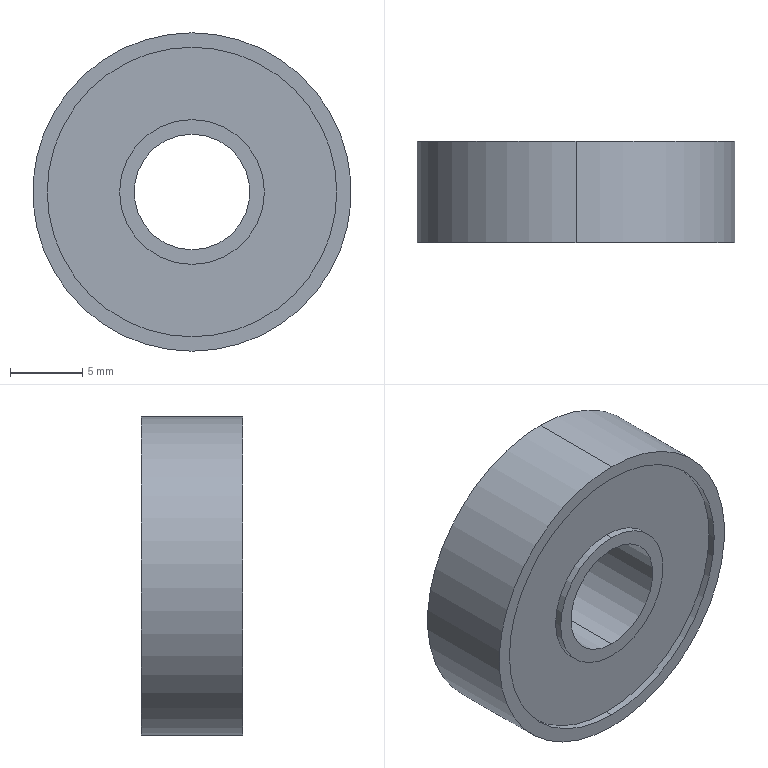Part | SolidWorks | features ICE 2, Extrusion 1 | 1 solid | 18 faces | box 22 x 7 x 22 mm | volume 2073 mm3 | cylinder 12 | plane 6 | commonest cylinder face diameters 10 x4 20 x4 8 x2 22 x2
STEP:
#1=CARTESIAN_POINT('',(0.,6.5,5.));
#2=VERTEX_POINT('',#1);
#3=CARTESIAN_POINT('',(0.,6.5,-5.));
#4=VERTEX_POINT('',#3);
#5=CARTESIAN_POINT('',(0.,6.5,0.));
#6=DIRECTION('',(0.,1.,0.));
#7=DIRECTION('',(0.,0.,1.));
#8=AXIS2_PLACEMENT_3D('',#5,#6,#7);
#9=CIRCLE('',#8,5.);
#10=EDGE_CURVE('',#2,#4,#9,.T.);
#11=ORIENTED_EDGE('',*,*,#10,.T.);
#12=CARTESIAN_POINT('',(0.,7.,-5.));
#13=VERTEX_POINT('',#12);
#14=CARTESIAN_POINT('',(0.,6.5,-5.));
#15=DIRECTION('',(0.,1.,0.));
#16=VECTOR('',#15,1000.);
#17=LINE('',#14,#16);
#18=EDGE_CURVE('',#4,#13,#17,.T.);
#19=ORIENTED_EDGE('',*,*,#18,.T.);
#20=CARTESIAN_POINT('',(0.,7.,5.));
#21=VERTEX_POINT('',#20);
#22=CARTESIAN_POINT('',(0.,7.,0.));
#23=DIRECTION('',(0.,1.,0.));
#24=DIRECTION('',(0.,0.,1.));
#25=AXIS2_PLACEMENT_3D('',#22,#23,#24);
#26=CIRCLE('',#25,5.);
#27=EDGE_CURVE('',#21,#13,#26,.T.);
#28=ORIENTED_EDGE('',*,*,#27,.F.);
#29=CARTESIAN_POINT('',(0.,6.5,5.));
#30=DIRECTION('',(0.,1.,0.));
#31=VECTOR('',#30,1000.);
#32=LINE('',#29,#31);
#33=EDGE_CURVE('',#2,#21,#32,.T.);
#34=ORIENTED_EDGE('',*,*,#33,.F.);
#35=EDGE_LOOP('',(#11,#19,#28,#34));
#36=FACE_OUTER_BOUND('',#35,.T.);
#37=CARTESIAN_POINT('',(0.,6.5,0.));
#38=DIRECTION('',(0.,1.,0.));
#39=DIRECTION('',(0.,0.,1.));
#40=AXIS2_PLACEMENT_3D('',#37,#38,#39);
#41=CYLINDRICAL_SURFACE('',#40,5.);
#42=ADVANCED_FACE('',(#36),#41,.T.);
#43=CARTESIAN_POINT('',(0.,6.5,-10.));
#44=VERTEX_POINT('',#43);
#45=CARTESIAN_POINT('',(0.,6.5,10.));
#46=VERTEX_POINT('',#45);
#47=CARTESIAN_POINT('',(0.,6.5,0.));
#48=DIRECTION('',(0.,1.,0.));
#49=DIRECTION('',(0.,0.,1.));
#50=AXIS2_PLACEMENT_3D('',#47,#48,#49);
#51=CIRCLE('',#50,10.);
#52=EDGE_CURVE('',#44,#46,#51,.T.);
#53=ORIENTED_EDGE('',*,*,#52,.F.);
#54=CARTESIAN_POINT('',(0.,7.,-10.));
#55=VERTEX_POINT('',#54);
#56=CARTESIAN_POINT('',(0.,6.5,-10.));
#57=DIRECTION('',(0.,1.,0.));
#58=VECTOR('',#57,1000.);
#59=LINE('',#56,#58);
#60=EDGE_CURVE('',#44,#55,#59,.T.);
#61=ORIENTED_EDGE('',*,*,#60,.T.);
#62=CARTESIAN_POINT('',(0.,7.,10.));
#63=VERTEX_POINT('',#62);
#64=CARTESIAN_POINT('',(0.,7.,0.));
#65=DIRECTION('',(0.,1.,0.));
#66=DIRECTION('',(0.,0.,1.));
#67=AXIS2_PLACEMENT_3D('',#64,#65,#66);
#68=CIRCLE('',#67,10.);
#69=EDGE_CURVE('',#55,#63,#68,.T.);
#70=ORIENTED_EDGE('',*,*,#69,.T.);
#71=CARTESIAN_POINT('',(0.,6.5,10.));
#72=DIRECTION('',(0.,1.,0.));
#73=VECTOR('',#72,1000.);
#74=LINE('',#71,#73);
#75=EDGE_CURVE('',#46,#63,#74,.T.);
#76=ORIENTED_EDGE('',*,*,#75,.F.);
#77=EDGE_LOOP('',(#53,#61,#70,#76));
#78=FACE_OUTER_BOUND('',#77,.T.);
#79=CARTESIAN_POINT('',(0.,6.5,0.));
#80=DIRECTION('',(0.,1.,0.));
#81=DIRECTION('',(0.,0.,1.));
#82=AXIS2_PLACEMENT_3D('',#79,#80,#81);
#83=CYLINDRICAL_SURFACE('',#82,10.);
#84=ADVANCED_FACE('',(#78),#83,.F.);
#85=CARTESIAN_POINT('',(0.,0.5,-5.));
#86=VERTEX_POINT('',#85);
#87=CARTESIAN_POINT('',(0.,0.5,5.));
#88=VERTEX_POINT('',#87);
#89=CARTESIAN_POINT('',(0.,0.5,0.));
#90=DIRECTION('',(0.,-1.,0.));
#91=DIRECTION('',(0.,0.,-1.));
#92=AXIS2_PLACEMENT_3D('',#89,#90,#91);
#93=CIRCLE('',#92,5.);
#94=EDGE_CURVE('',#86,#88,#93,.T.);
#95=ORIENTED_EDGE('',*,*,#94,.T.);
#96=CARTESIAN_POINT('',(0.,0.,5.));
#97=VERTEX_POINT('',#96);
#98=CARTESIAN_POINT('',(0.,0.5,5.));
#99=DIRECTION('',(0.,-1.,0.));
#100=VECTOR('',#99,1000.);
#101=LINE('',#98,#100);
#102=EDGE_CURVE('',#88,#97,#101,.T.);
#103=ORIENTED_EDGE('',*,*,#102,.T.);
#104=CARTESIAN_POINT('',(0.,0.,-5.));
#105=VERTEX_POINT('',#104);
#106=CARTESIAN_POINT('',(0.,0.,0.));
#107=DIRECTION('',(0.,-1.,0.));
#108=DIRECTION('',(0.,0.,-1.));
#109=AXIS2_PLACEMENT_3D('',#106,#107,#108);
#110=CIRCLE('',#109,5.);
#111=EDGE_CURVE('',#105,#97,#110,.T.);
#112=ORIENTED_EDGE('',*,*,#111,.F.);
#113=CARTESIAN_POINT('',(0.,0.5,-5.));
#114=DIRECTION('',(0.,-1.,0.));
#115=VECTOR('',#114,1000.);
#116=LINE('',#113,#115);
#117=EDGE_CURVE('',#86,#105,#116,.T.);
#118=ORIENTED_EDGE('',*,*,#117,.F.);
#119=EDGE_LOOP('',(#95,#103,#112,#118));
#120=FACE_OUTER_BOUND('',#119,.T.);
#121=CARTESIAN_POINT('',(0.,0.5,0.));
#122=DIRECTION('',(0.,-1.,0.));
#123=DIRECTION('',(0.,0.,-1.));
#124=AXIS2_PLACEMENT_3D('',#121,#122,#123);
#125=CYLINDRICAL_SURFACE('',#124,5.);
#126=ADVANCED_FACE('',(#120),#125,.T.);
#127=CARTESIAN_POINT('',(0.,0.5,10.));
#128=VERTEX_POINT('',#127);
#129=CARTESIAN_POINT('',(0.,0.5,-10.));
#130=VERTEX_POINT('',#129);
#131=CARTESIAN_POINT('',(0.,0.5,0.));
#132=DIRECTION('',(0.,-1.,0.));
#133=DIRECTION('',(0.,0.,-1.));
#134=AXIS2_PLACEMENT_3D('',#131,#132,#133);
#135=CIRCLE('',#134,10.);
#136=EDGE_CURVE('',#128,#130,#135,.T.);
#137=ORIENTED_EDGE('',*,*,#136,.F.);
#138=CARTESIAN_POINT('',(0.,0.,10.));
#139=VERTEX_POINT('',#138);
#140=CARTESIAN_POINT('',(0.,0.5,10.));
#141=DIRECTION('',(0.,-1.,0.));
#142=VECTOR('',#141,1000.);
#143=LINE('',#140,#142);
#144=EDGE_CURVE('',#128,#139,#143,.T.);
#145=ORIENTED_EDGE('',*,*,#144,.T.);
#146=CARTESIAN_POINT('',(0.,0.,-10.));
#147=VERTEX_POINT('',#146);
#148=CARTESIAN_POINT('',(0.,0.,0.));
#149=DIRECTION('',(0.,-1.,0.));
#150=DIRECTION('',(0.,0.,-1.));
#151=AXIS2_PLACEMENT_3D('',#148,#149,#150);
#152=CIRCLE('',#151,10.);
#153=EDGE_CURVE('',#139,#147,#152,.T.);
#154=ORIENTED_EDGE('',*,*,#153,.T.);
#155=CARTESIAN_POINT('',(0.,0.5,-10.));
#156=DIRECTION('',(0.,-1.,0.));
#157=VECTOR('',#156,1000.);
#158=LINE('',#155,#157);
#159=EDGE_CURVE('',#130,#147,#158,.T.);
#160=ORIENTED_EDGE('',*,*,#159,.F.);
#161=EDGE_LOOP('',(#137,#145,#154,#160));
#162=FACE_OUTER_BOUND('',#161,.T.);
#163=CARTESIAN_POINT('',(0.,0.5,0.));
#164=DIRECTION('',(0.,-1.,0.));
#165=DIRECTION('',(0.,0.,-1.));
#166=AXIS2_PLACEMENT_3D('',#163,#164,#165);
#167=CYLINDRICAL_SURFACE('',#166,10.);
#168=ADVANCED_FACE('',(#162),#167,.F.);
#169=CARTESIAN_POINT('',(0.,7.,-4.));
#170=VERTEX_POINT('',#169);
#171=CARTESIAN_POINT('',(0.,7.,4.));
#172=VERTEX_POINT('',#171);
#173=CARTESIAN_POINT('',(0.,7.,0.));
#174=DIRECTION('',(0.,1.,0.));
#175=DIRECTION('',(0.,0.,1.));
#176=AXIS2_PLACEMENT_3D('',#173,#174,#175);
#177=CIRCLE('',#176,4.);
#178=EDGE_CURVE('',#170,#172,#177,.T.);
#179=ORIENTED_EDGE('',*,*,#178,.T.);
#180=CARTESIAN_POINT('',(0.,0.,4.));
#181=VERTEX_POINT('',#180);
#182=CARTESIAN_POINT('',(0.,7.,4.));
#183=DIRECTION('',(0.,-1.,0.));
#184=VECTOR('',#183,1000.);
#185=LINE('',#182,#184);
#186=EDGE_CURVE('',#172,#181,#185,.T.);
#187=ORIENTED_EDGE('',*,*,#186,.T.);
#188=CARTESIAN_POINT('',(0.,0.,-4.));
#189=VERTEX_POINT('',#188);
#190=CARTESIAN_POINT('',(0.,0.,0.));
#191=DIRECTION('',(0.,1.,0.));
#192=DIRECTION('',(0.,0.,1.));
#193=AXIS2_PLACEMENT_3D('',#190,#191,#192);
#194=CIRCLE('',#193,4.);
#195=EDGE_CURVE('',#189,#181,#194,.T.);
#196=ORIENTED_EDGE('',*,*,#195,.F.);
#197=CARTESIAN_POINT('',(0.,7.,-4.));
#198=DIRECTION('',(0.,-1.,0.));
#199=VECTOR('',#198,1000.);
#200=LINE('',#197,#199);
#201=EDGE_CURVE('',#170,#189,#200,.T.);
#202=ORIENTED_EDGE('',*,*,#201,.F.);
#203=EDGE_LOOP('',(#179,#187,#196,#202));
#204=FACE_OUTER_BOUND('',#203,.T.);
#205=CARTESIAN_POINT('',(0.,7.,0.));
#206=DIRECTION('',(0.,-1.,0.));
#207=DIRECTION('',(0.,0.,-1.));
#208=AXIS2_PLACEMENT_3D('',#205,#206,#207);
#209=CYLINDRICAL_SURFACE('',#208,4.);
#210=ADVANCED_FACE('',(#204),#209,.F.);
#211=CARTESIAN_POINT('',(0.,7.,11.));
#212=VERTEX_POINT('',#211);
#213=CARTESIAN_POINT('',(0.,7.,-11.));
#214=VERTEX_POINT('',#213);
#215=CARTESIAN_POINT('',(0.,7.,0.));
#216=DIRECTION('',(0.,1.,0.));
#217=DIRECTION('',(0.,0.,1.));
#218=AXIS2_PLACEMENT_3D('',#215,#216,#217);
#219=CIRCLE('',#218,11.);
#220=EDGE_CURVE('',#212,#214,#219,.T.);
#221=ORIENTED_EDGE('',*,*,#220,.F.);
#222=CARTESIAN_POINT('',(0.,0.,11.));
#223=VERTEX_POINT('',#222);
#224=CARTESIAN_POINT('',(0.,7.,11.));
#225=DIRECTION('',(0.,-1.,0.));
#226=VECTOR('',#225,1000.);
#227=LINE('',#224,#226);
#228=EDGE_CURVE('',#212,#223,#227,.T.);
#229=ORIENTED_EDGE('',*,*,#228,.T.);
#230=CARTESIAN_POINT('',(0.,0.,-11.));
#231=VERTEX_POINT('',#230);
#232=CARTESIAN_POINT('',(0.,0.,0.));
#233=DIRECTION('',(0.,1.,0.));
#234=DIRECTION('',(0.,0.,1.));
#235=AXIS2_PLACEMENT_3D('',#232,#233,#234);
#236=CIRCLE('',#235,11.);
#237=EDGE_CURVE('',#223,#231,#236,.T.);
#238=ORIENTED_EDGE('',*,*,#237,.T.);
#239=CARTESIAN_POINT('',(0.,7.,-11.));
#240=DIRECTION('',(0.,-1.,0.));
#241=VECTOR('',#240,1000.);
#242=LINE('',#239,#241);
#243=EDGE_CURVE('',#214,#231,#242,.T.);
#244=ORIENTED_EDGE('',*,*,#243,.F.);
#245=EDGE_LOOP('',(#221,#229,#238,#244));
#246=FACE_OUTER_BOUND('',#245,.T.);
#247=CARTESIAN_POINT('',(0.,7.,0.));
#248=DIRECTION('',(0.,-1.,0.));
#249=DIRECTION('',(0.,0.,-1.));
#250=AXIS2_PLACEMENT_3D('',#247,#248,#249);
#251=CYLINDRICAL_SURFACE('',#250,11.);
#252=ADVANCED_FACE('',(#246),#251,.T.);
#253=ORIENTED_EDGE('',*,*,#178,.F.);
#254=CARTESIAN_POINT('',(0.,7.,0.));
#255=DIRECTION('',(0.,1.,0.));
#256=DIRECTION('',(0.,0.,1.));
#257=AXIS2_PLACEMENT_3D('',#254,#255,#256);
#258=CIRCLE('',#257,4.);
#259=EDGE_CURVE('',#172,#170,#258,.T.);
#260=ORIENTED_EDGE('',*,*,#259,.F.);
#261=EDGE_LOOP('',(#253,#260));
#262=FACE_BOUND('',#261,.T.);
#263=ORIENTED_EDGE('',*,*,#27,.T.);
#264=CARTESIAN_POINT('',(0.,7.,0.));
#265=DIRECTION('',(0.,1.,0.));
#266=DIRECTION('',(0.,0.,1.));
#267=AXIS2_PLACEMENT_3D('',#264,#265,#266);
#268=CIRCLE('',#267,5.);
#269=EDGE_CURVE('',#13,#21,#268,.T.);
#270=ORIENTED_EDGE('',*,*,#269,.T.);
#271=EDGE_LOOP('',(#263,#270));
#272=FACE_OUTER_BOUND('',#271,.T.);
#273=CARTESIAN_POINT('',(0.,7.,0.));
#274=DIRECTION('',(0.,1.,0.));
#275=DIRECTION('',(0.,0.,1.));
#276=AXIS2_PLACEMENT_3D('',#273,#274,#275);
#277=PLANE('',#276);
#278=ADVANCED_FACE('',(#262,#272),#277,.T.);
#279=ORIENTED_EDGE('',*,*,#195,.T.);
#280=CARTESIAN_POINT('',(0.,0.,0.));
#281=DIRECTION('',(0.,1.,0.));
#282=DIRECTION('',(0.,0.,1.));
#283=AXIS2_PLACEMENT_3D('',#280,#281,#282);
#284=CIRCLE('',#283,4.);
#285=EDGE_CURVE('',#181,#189,#284,.T.);
#286=ORIENTED_EDGE('',*,*,#285,.T.);
#287=EDGE_LOOP('',(#279,#286));
#288=FACE_BOUND('',#287,.T.);
#289=ORIENTED_EDGE('',*,*,#111,.T.);
#290=CARTESIAN_POINT('',(0.,0.,0.));
#291=DIRECTION('',(0.,-1.,0.));
#292=DIRECTION('',(0.,0.,-1.));
#293=AXIS2_PLACEMENT_3D('',#290,#291,#292);
#294=CIRCLE('',#293,5.);
#295=EDGE_CURVE('',#97,#105,#294,.T.);
#296=ORIENTED_EDGE('',*,*,#295,.T.);
#297=EDGE_LOOP('',(#289,#296));
#298=FACE_OUTER_BOUND('',#297,.T.);
#299=CARTESIAN_POINT('',(0.,0.,0.));
#300=DIRECTION('',(0.,1.,0.));
#301=DIRECTION('',(0.,0.,1.));
#302=AXIS2_PLACEMENT_3D('',#299,#300,#301);
#303=PLANE('',#302);
#304=ADVANCED_FACE('',(#288,#298),#303,.F.);
#305=CARTESIAN_POINT('',(0.,7.,0.));
#306=DIRECTION('',(0.,1.,0.));
#307=DIRECTION('',(0.,0.,1.));
#308=AXIS2_PLACEMENT_3D('',#305,#306,#307);
#309=CIRCLE('',#308,10.);
#310=EDGE_CURVE('',#63,#55,#309,.T.);
#311=ORIENTED_EDGE('',*,*,#310,.F.);
#312=ORIENTED_EDGE('',*,*,#69,.F.);
#313=EDGE_LOOP('',(#311,#312));
#314=FACE_BOUND('',#313,.T.);
#315=CARTESIAN_POINT('',(0.,7.,0.));
#316=DIRECTION('',(0.,1.,0.));
#317=DIRECTION('',(0.,0.,1.));
#318=AXIS2_PLACEMENT_3D('',#315,#316,#317);
#319=CIRCLE('',#318,11.);
#320=EDGE_CURVE('',#214,#212,#319,.T.);
#321=ORIENTED_EDGE('',*,*,#320,.T.);
#322=ORIENTED_EDGE('',*,*,#220,.T.);
#323=EDGE_LOOP('',(#321,#322));
#324=FACE_OUTER_BOUND('',#323,.T.);
#325=CARTESIAN_POINT('',(0.,7.,0.));
#326=DIRECTION('',(0.,1.,0.));
#327=DIRECTION('',(0.,0.,1.));
#328=AXIS2_PLACEMENT_3D('',#325,#326,#327);
#329=PLANE('',#328);
#330=ADVANCED_FACE('',(#314,#324),#329,.T.);
#331=CARTESIAN_POINT('',(0.,0.,0.));
#332=DIRECTION('',(0.,-1.,0.));
#333=DIRECTION('',(0.,0.,-1.));
#334=AXIS2_PLACEMENT_3D('',#331,#332,#333);
#335=CIRCLE('',#334,10.);
#336=EDGE_CURVE('',#147,#139,#335,.T.);
#337=ORIENTED_EDGE('',*,*,#336,.F.);
#338=ORIENTED_EDGE('',*,*,#153,.F.);
#339=EDGE_LOOP('',(#337,#338));
#340=FACE_BOUND('',#339,.T.);
#341=CARTESIAN_POINT('',(0.,0.,0.));
#342=DIRECTION('',(0.,1.,0.));
#343=DIRECTION('',(0.,0.,1.));
#344=AXIS2_PLACEMENT_3D('',#341,#342,#343);
#345=CIRCLE('',#344,11.);
#346=EDGE_CURVE('',#231,#223,#345,.T.);
#347=ORIENTED_EDGE('',*,*,#346,.F.);
#348=ORIENTED_EDGE('',*,*,#237,.F.);
#349=EDGE_LOOP('',(#347,#348));
#350=FACE_OUTER_BOUND('',#349,.T.);
#351=CARTESIAN_POINT('',(0.,0.,0.));
#352=DIRECTION('',(0.,1.,0.));
#353=DIRECTION('',(0.,0.,1.));
#354=AXIS2_PLACEMENT_3D('',#351,#352,#353);
#355=PLANE('',#354);
#356=ADVANCED_FACE('',(#340,#350),#355,.F.);
#357=ORIENTED_EDGE('',*,*,#228,.F.);
#358=ORIENTED_EDGE('',*,*,#320,.F.);
#359=ORIENTED_EDGE('',*,*,#243,.T.);
#360=ORIENTED_EDGE('',*,*,#346,.T.);
#361=EDGE_LOOP('',(#357,#358,#359,#360));
#362=FACE_OUTER_BOUND('',#361,.T.);
#363=CARTESIAN_POINT('',(0.,7.,0.));
#364=DIRECTION('',(0.,-1.,0.));
#365=DIRECTION('',(0.,0.,-1.));
#366=AXIS2_PLACEMENT_3D('',#363,#364,#365);
#367=CYLINDRICAL_SURFACE('',#366,11.);
#368=ADVANCED_FACE('',(#362),#367,.T.);
#369=ORIENTED_EDGE('',*,*,#186,.F.);
#370=ORIENTED_EDGE('',*,*,#259,.T.);
#371=ORIENTED_EDGE('',*,*,#201,.T.);
#372=ORIENTED_EDGE('',*,*,#285,.F.);
#373=EDGE_LOOP('',(#369,#370,#371,#372));
#374=FACE_OUTER_BOUND('',#373,.T.);
#375=CARTESIAN_POINT('',(0.,7.,0.));
#376=DIRECTION('',(0.,-1.,0.));
#377=DIRECTION('',(0.,0.,-1.));
#378=AXIS2_PLACEMENT_3D('',#375,#376,#377);
#379=CYLINDRICAL_SURFACE('',#378,4.);
#380=ADVANCED_FACE('',(#374),#379,.F.);
#381=ORIENTED_EDGE('',*,*,#144,.F.);
#382=CARTESIAN_POINT('',(0.,0.5,0.));
#383=DIRECTION('',(0.,-1.,0.));
#384=DIRECTION('',(0.,0.,-1.));
#385=AXIS2_PLACEMENT_3D('',#382,#383,#384);
#386=CIRCLE('',#385,10.);
#387=EDGE_CURVE('',#130,#128,#386,.T.);
#388=ORIENTED_EDGE('',*,*,#387,.F.);
#389=ORIENTED_EDGE('',*,*,#159,.T.);
#390=ORIENTED_EDGE('',*,*,#336,.T.);
#391=EDGE_LOOP('',(#381,#388,#389,#390));
#392=FACE_OUTER_BOUND('',#391,.T.);
#393=CARTESIAN_POINT('',(0.,0.5,0.));
#394=DIRECTION('',(0.,-1.,0.));
#395=DIRECTION('',(0.,0.,-1.));
#396=AXIS2_PLACEMENT_3D('',#393,#394,#395);
#397=CYLINDRICAL_SURFACE('',#396,10.);
#398=ADVANCED_FACE('',(#392),#397,.F.);
#399=ORIENTED_EDGE('',*,*,#94,.F.);
#400=CARTESIAN_POINT('',(0.,0.5,0.));
#401=DIRECTION('',(0.,-1.,0.));
#402=DIRECTION('',(0.,0.,-1.));
#403=AXIS2_PLACEMENT_3D('',#400,#401,#402);
#404=CIRCLE('',#403,5.);
#405=EDGE_CURVE('',#88,#86,#404,.T.);
#406=ORIENTED_EDGE('',*,*,#405,.F.);
#407=EDGE_LOOP('',(#399,#406));
#408=FACE_BOUND('',#407,.T.);
#409=ORIENTED_EDGE('',*,*,#387,.T.);
#410=ORIENTED_EDGE('',*,*,#136,.T.);
#411=EDGE_LOOP('',(#409,#410));
#412=FACE_OUTER_BOUND('',#411,.T.);
#413=CARTESIAN_POINT('',(0.,0.5,0.));
#414=DIRECTION('',(0.,-1.,0.));
#415=DIRECTION('',(0.,0.,-1.));
#416=AXIS2_PLACEMENT_3D('',#413,#414,#415);
#417=PLANE('',#416);
#418=ADVANCED_FACE('',(#408,#412),#417,.T.);
#419=ORIENTED_EDGE('',*,*,#102,.F.);
#420=ORIENTED_EDGE('',*,*,#405,.T.);
#421=ORIENTED_EDGE('',*,*,#117,.T.);
#422=ORIENTED_EDGE('',*,*,#295,.F.);
#423=EDGE_LOOP('',(#419,#420,#421,#422));
#424=FACE_OUTER_BOUND('',#423,.T.);
#425=CARTESIAN_POINT('',(0.,0.5,0.));
#426=DIRECTION('',(0.,-1.,0.));
#427=DIRECTION('',(0.,0.,-1.));
#428=AXIS2_PLACEMENT_3D('',#425,#426,#427);
#429=CYLINDRICAL_SURFACE('',#428,5.);
#430=ADVANCED_FACE('',(#424),#429,.T.);
#431=ORIENTED_EDGE('',*,*,#60,.F.);
#432=CARTESIAN_POINT('',(0.,6.5,0.));
#433=DIRECTION('',(0.,1.,0.));
#434=DIRECTION('',(0.,0.,1.));
#435=AXIS2_PLACEMENT_3D('',#432,#433,#434);
#436=CIRCLE('',#435,10.);
#437=EDGE_CURVE('',#46,#44,#436,.T.);
#438=ORIENTED_EDGE('',*,*,#437,.F.);
#439=ORIENTED_EDGE('',*,*,#75,.T.);
#440=ORIENTED_EDGE('',*,*,#310,.T.);
#441=EDGE_LOOP('',(#431,#438,#439,#440));
#442=FACE_OUTER_BOUND('',#441,.T.);
#443=CARTESIAN_POINT('',(0.,6.5,0.));
#444=DIRECTION('',(0.,1.,0.));
#445=DIRECTION('',(0.,0.,1.));
#446=AXIS2_PLACEMENT_3D('',#443,#444,#445);
#447=CYLINDRICAL_SURFACE('',#446,10.);
#448=ADVANCED_FACE('',(#442),#447,.F.);
#449=ORIENTED_EDGE('',*,*,#10,.F.);
#450=CARTESIAN_POINT('',(0.,6.5,0.));
#451=DIRECTION('',(0.,1.,0.));
#452=DIRECTION('',(0.,0.,1.));
#453=AXIS2_PLACEMENT_3D('',#450,#451,#452);
#454=CIRCLE('',#453,5.);
#455=EDGE_CURVE('',#4,#2,#454,.T.);
#456=ORIENTED_EDGE('',*,*,#455,.F.);
#457=EDGE_LOOP('',(#449,#456));
#458=FACE_BOUND('',#457,.T.);
#459=ORIENTED_EDGE('',*,*,#437,.T.);
#460=ORIENTED_EDGE('',*,*,#52,.T.);
#461=EDGE_LOOP('',(#459,#460));
#462=FACE_OUTER_BOUND('',#461,.T.);
#463=CARTESIAN_POINT('',(0.,6.5,0.));
#464=DIRECTION('',(0.,1.,0.));
#465=DIRECTION('',(0.,0.,1.));
#466=AXIS2_PLACEMENT_3D('',#463,#464,#465);
#467=PLANE('',#466);
#468=ADVANCED_FACE('',(#458,#462),#467,.T.);
#469=ORIENTED_EDGE('',*,*,#18,.F.);
#470=ORIENTED_EDGE('',*,*,#455,.T.);
#471=ORIENTED_EDGE('',*,*,#33,.T.);
#472=ORIENTED_EDGE('',*,*,#269,.F.);
#473=EDGE_LOOP('',(#469,#470,#471,#472));
#474=FACE_OUTER_BOUND('',#473,.T.);
#475=CARTESIAN_POINT('',(0.,6.5,0.));
#476=DIRECTION('',(0.,1.,0.));
#477=DIRECTION('',(0.,0.,1.));
#478=AXIS2_PLACEMENT_3D('',#475,#476,#477);
#479=CYLINDRICAL_SURFACE('',#478,5.);
#480=ADVANCED_FACE('',(#474),#479,.T.);
#481=CLOSED_SHELL('',(#42,#84,#126,#168,#210,#252,#278,#304,#330,#356,#368,#380,#398,#418,#430,#448,#468,#480));
#482=MANIFOLD_SOLID_BREP('',#481);
#483=CARTESIAN_POINT('',(0.,0.,0.));
#484=DIRECTION('',(0.,0.,1.));
#485=DIRECTION('',(1.,0.,0.));
#486=AXIS2_PLACEMENT_3D('',#483,#484,#485);
#487=(LENGTH_UNIT()NAMED_UNIT(*)SI_UNIT(.MILLI.,.METRE.));
#488=UNCERTAINTY_MEASURE_WITH_UNIT(LENGTH_MEASURE(0.00001),#487,'','');
#489=(NAMED_UNIT(*)PLANE_ANGLE_UNIT()SI_UNIT($,.RADIAN.));
#490=(NAMED_UNIT(*)SI_UNIT($,.STERADIAN.)SOLID_ANGLE_UNIT());
#491=(GEOMETRIC_REPRESENTATION_CONTEXT(3)GLOBAL_UNCERTAINTY_ASSIGNED_CONTEXT((#488))GLOBAL_UNIT_ASSIGNED_CONTEXT((#487,#489,#490))REPRESENTATION_CONTEXT('',''));
#492=ADVANCED_BREP_SHAPE_REPRESENTATION('',(#482,#486),#491);